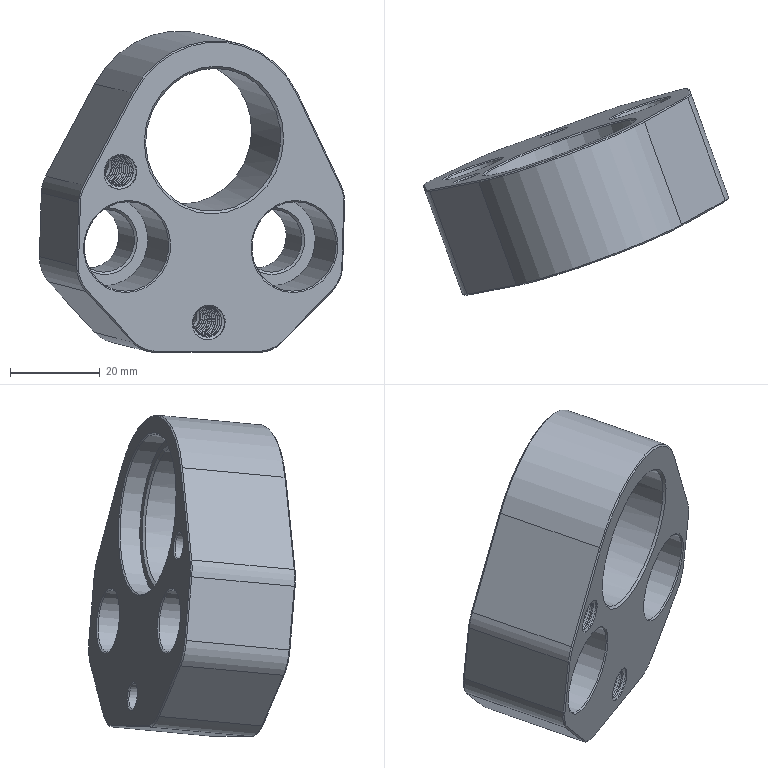Part | NX | features solid 2 | 1 solid | 82 faces | box 67.946 x 46.06 x 71.561 mm | volume 50954 mm3 | plane 30 | cone 29 | cylinder 19 | spline 4 | commonest cylinder face diameters 16 x6 5.8 x2 6.918 x2 8 x2 14 x2 20 x2